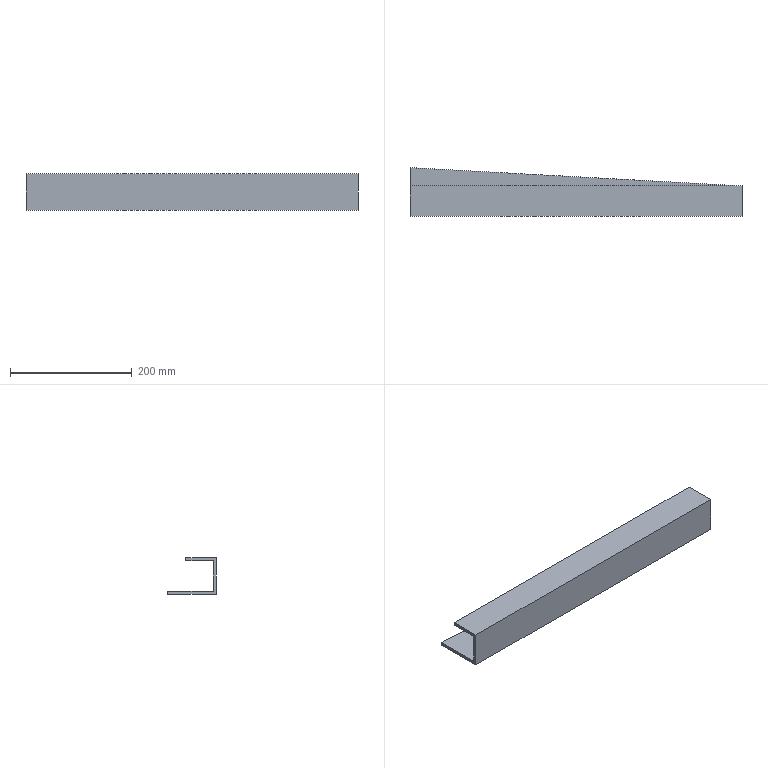Part | SolidWorks | features Extrusion 1, ICE 1, Shell 1 | 1 solid | 10 faces | box 545 x 80 x 60 mm | volume 449625 mm3 | plane 10
STEP:
#1=CARTESIAN_POINT('',(545.,-30.,5.));
#2=VERTEX_POINT('',#1);
#3=CARTESIAN_POINT('',(0.,0.,5.));
#4=VERTEX_POINT('',#3);
#5=CARTESIAN_POINT('',(545.,-30.,5.));
#6=DIRECTION('',(-0.9985,0.05496,0.));
#7=VECTOR('',#6,1000.);
#8=LINE('',#5,#7);
#9=EDGE_CURVE('',#2,#4,#8,.T.);
#10=ORIENTED_EDGE('',*,*,#9,.F.);
#11=CARTESIAN_POINT('',(545.,-30.,0.));
#12=VERTEX_POINT('',#11);
#13=CARTESIAN_POINT('',(545.,-30.,60.));
#14=DIRECTION('',(0.,0.,-1.));
#15=VECTOR('',#14,1000.);
#16=LINE('',#13,#15);
#17=EDGE_CURVE('',#2,#12,#16,.T.);
#18=ORIENTED_EDGE('',*,*,#17,.T.);
#19=CARTESIAN_POINT('',(0.,0.,0.));
#20=VERTEX_POINT('',#19);
#21=CARTESIAN_POINT('',(545.,-30.,0.));
#22=DIRECTION('',(-0.9985,0.05496,0.));
#23=VECTOR('',#22,1000.);
#24=LINE('',#21,#23);
#25=EDGE_CURVE('',#12,#20,#24,.T.);
#26=ORIENTED_EDGE('',*,*,#25,.T.);
#27=CARTESIAN_POINT('',(0.,0.,60.));
#28=DIRECTION('',(0.,0.,-1.));
#29=VECTOR('',#28,1000.);
#30=LINE('',#27,#29);
#31=EDGE_CURVE('',#4,#20,#30,.T.);
#32=ORIENTED_EDGE('',*,*,#31,.F.);
#33=EDGE_LOOP('',(#10,#18,#26,#32));
#34=FACE_OUTER_BOUND('',#33,.T.);
#35=CARTESIAN_POINT('',(545.,-30.,60.));
#36=DIRECTION('',(-0.05496,-0.9985,0.));
#37=DIRECTION('',(0.9985,-0.05496,0.));
#38=AXIS2_PLACEMENT_3D('',#35,#36,#37);
#39=PLANE('',#38);
#40=ADVANCED_FACE('',(#34),#39,.F.);
#41=CARTESIAN_POINT('',(0.,-30.,60.));
#42=VERTEX_POINT('',#41);
#43=CARTESIAN_POINT('',(0.,-80.,60.));
#44=VERTEX_POINT('',#43);
#45=CARTESIAN_POINT('',(0.,0.,60.));
#46=DIRECTION('',(0.,-1.,0.));
#47=VECTOR('',#46,1000.);
#48=LINE('',#45,#47);
#49=EDGE_CURVE('',#42,#44,#48,.T.);
#50=ORIENTED_EDGE('',*,*,#49,.F.);
#51=CARTESIAN_POINT('',(0.,-30.,55.));
#52=VERTEX_POINT('',#51);
#53=CARTESIAN_POINT('',(0.,-30.,22.));
#54=DIRECTION('',(0.,0.,1.));
#55=VECTOR('',#54,1000.);
#56=LINE('',#53,#55);
#57=EDGE_CURVE('',#52,#42,#56,.T.);
#58=ORIENTED_EDGE('',*,*,#57,.F.);
#59=CARTESIAN_POINT('',(0.,-75.,55.));
#60=VERTEX_POINT('',#59);
#61=CARTESIAN_POINT('',(0.,0.,55.));
#62=DIRECTION('',(0.,-1.,0.));
#63=VECTOR('',#62,1000.);
#64=LINE('',#61,#63);
#65=EDGE_CURVE('',#52,#60,#64,.T.);
#66=ORIENTED_EDGE('',*,*,#65,.T.);
#67=CARTESIAN_POINT('',(0.,-75.,5.));
#68=VERTEX_POINT('',#67);
#69=CARTESIAN_POINT('',(0.,-75.,60.));
#70=DIRECTION('',(0.,0.,-1.));
#71=VECTOR('',#70,1000.);
#72=LINE('',#69,#71);
#73=EDGE_CURVE('',#60,#68,#72,.T.);
#74=ORIENTED_EDGE('',*,*,#73,.T.);
#75=CARTESIAN_POINT('',(0.,0.,5.));
#76=DIRECTION('',(0.,-1.,0.));
#77=VECTOR('',#76,1000.);
#78=LINE('',#75,#77);
#79=EDGE_CURVE('',#4,#68,#78,.T.);
#80=ORIENTED_EDGE('',*,*,#79,.F.);
#81=ORIENTED_EDGE('',*,*,#31,.T.);
#82=CARTESIAN_POINT('',(0.,-80.,0.));
#83=VERTEX_POINT('',#82);
#84=CARTESIAN_POINT('',(0.,0.,0.));
#85=DIRECTION('',(0.,-1.,0.));
#86=VECTOR('',#85,1000.);
#87=LINE('',#84,#86);
#88=EDGE_CURVE('',#20,#83,#87,.T.);
#89=ORIENTED_EDGE('',*,*,#88,.T.);
#90=CARTESIAN_POINT('',(0.,-80.,60.));
#91=DIRECTION('',(0.,0.,-1.));
#92=VECTOR('',#91,1000.);
#93=LINE('',#90,#92);
#94=EDGE_CURVE('',#44,#83,#93,.T.);
#95=ORIENTED_EDGE('',*,*,#94,.F.);
#96=EDGE_LOOP('',(#50,#58,#66,#74,#80,#81,#89,#95));
#97=FACE_OUTER_BOUND('',#96,.T.);
#98=CARTESIAN_POINT('',(0.,0.,60.));
#99=DIRECTION('',(1.,0.,0.));
#100=DIRECTION('',(0.,1.,0.));
#101=AXIS2_PLACEMENT_3D('',#98,#99,#100);
#102=PLANE('',#101);
#103=ADVANCED_FACE('',(#97),#102,.F.);
#104=CARTESIAN_POINT('',(545.,-75.,5.));
#105=VERTEX_POINT('',#104);
#106=CARTESIAN_POINT('',(545.,-80.,5.));
#107=DIRECTION('',(0.,1.,0.));
#108=VECTOR('',#107,1000.);
#109=LINE('',#106,#108);
#110=EDGE_CURVE('',#105,#2,#109,.T.);
#111=ORIENTED_EDGE('',*,*,#110,.F.);
#112=CARTESIAN_POINT('',(545.,-75.,55.));
#113=VERTEX_POINT('',#112);
#114=CARTESIAN_POINT('',(545.,-75.,60.));
#115=DIRECTION('',(0.,0.,-1.));
#116=VECTOR('',#115,1000.);
#117=LINE('',#114,#116);
#118=EDGE_CURVE('',#113,#105,#117,.T.);
#119=ORIENTED_EDGE('',*,*,#118,.F.);
#120=CARTESIAN_POINT('',(545.,-30.,55.));
#121=VERTEX_POINT('',#120);
#122=CARTESIAN_POINT('',(545.,-80.,55.));
#123=DIRECTION('',(0.,1.,0.));
#124=VECTOR('',#123,1000.);
#125=LINE('',#122,#124);
#126=EDGE_CURVE('',#113,#121,#125,.T.);
#127=ORIENTED_EDGE('',*,*,#126,.T.);
#128=CARTESIAN_POINT('',(545.,-30.,60.));
#129=VERTEX_POINT('',#128);
#130=CARTESIAN_POINT('',(545.,-30.,60.));
#131=DIRECTION('',(0.,0.,-1.));
#132=VECTOR('',#131,1000.);
#133=LINE('',#130,#132);
#134=EDGE_CURVE('',#129,#121,#133,.T.);
#135=ORIENTED_EDGE('',*,*,#134,.F.);
#136=CARTESIAN_POINT('',(545.,-80.,60.));
#137=VERTEX_POINT('',#136);
#138=CARTESIAN_POINT('',(545.,-80.,60.));
#139=DIRECTION('',(0.,1.,0.));
#140=VECTOR('',#139,1000.);
#141=LINE('',#138,#140);
#142=EDGE_CURVE('',#137,#129,#141,.T.);
#143=ORIENTED_EDGE('',*,*,#142,.F.);
#144=CARTESIAN_POINT('',(545.,-80.,0.));
#145=VERTEX_POINT('',#144);
#146=CARTESIAN_POINT('',(545.,-80.,60.));
#147=DIRECTION('',(0.,0.,-1.));
#148=VECTOR('',#147,1000.);
#149=LINE('',#146,#148);
#150=EDGE_CURVE('',#137,#145,#149,.T.);
#151=ORIENTED_EDGE('',*,*,#150,.T.);
#152=CARTESIAN_POINT('',(545.,-80.,0.));
#153=DIRECTION('',(0.,1.,0.));
#154=VECTOR('',#153,1000.);
#155=LINE('',#152,#154);
#156=EDGE_CURVE('',#145,#12,#155,.T.);
#157=ORIENTED_EDGE('',*,*,#156,.T.);
#158=ORIENTED_EDGE('',*,*,#17,.F.);
#159=EDGE_LOOP('',(#111,#119,#127,#135,#143,#151,#157,#158));
#160=FACE_OUTER_BOUND('',#159,.T.);
#161=CARTESIAN_POINT('',(545.,-80.,60.));
#162=DIRECTION('',(-1.,0.,0.));
#163=DIRECTION('',(0.,0.,1.));
#164=AXIS2_PLACEMENT_3D('',#161,#162,#163);
#165=PLANE('',#164);
#166=ADVANCED_FACE('',(#160),#165,.F.);
#167=CARTESIAN_POINT('',(0.,-80.,0.));
#168=DIRECTION('',(1.,0.,0.));
#169=VECTOR('',#168,1000.);
#170=LINE('',#167,#169);
#171=EDGE_CURVE('',#83,#145,#170,.T.);
#172=ORIENTED_EDGE('',*,*,#171,.T.);
#173=ORIENTED_EDGE('',*,*,#150,.F.);
#174=CARTESIAN_POINT('',(0.,-80.,60.));
#175=DIRECTION('',(1.,0.,0.));
#176=VECTOR('',#175,1000.);
#177=LINE('',#174,#176);
#178=EDGE_CURVE('',#44,#137,#177,.T.);
#179=ORIENTED_EDGE('',*,*,#178,.F.);
#180=ORIENTED_EDGE('',*,*,#94,.T.);
#181=EDGE_LOOP('',(#172,#173,#179,#180));
#182=FACE_OUTER_BOUND('',#181,.T.);
#183=CARTESIAN_POINT('',(0.,-80.,60.));
#184=DIRECTION('',(0.,1.,0.));
#185=DIRECTION('',(0.,0.,1.));
#186=AXIS2_PLACEMENT_3D('',#183,#184,#185);
#187=PLANE('',#186);
#188=ADVANCED_FACE('',(#182),#187,.F.);
#189=CARTESIAN_POINT('',(545.,-30.,60.));
#190=DIRECTION('',(1.,0.,0.));
#191=VECTOR('',#190,1000.);
#192=LINE('',#189,#191);
#193=EDGE_CURVE('',#42,#129,#192,.T.);
#194=ORIENTED_EDGE('',*,*,#193,.F.);
#195=ORIENTED_EDGE('',*,*,#49,.T.);
#196=ORIENTED_EDGE('',*,*,#178,.T.);
#197=ORIENTED_EDGE('',*,*,#142,.T.);
#198=EDGE_LOOP('',(#194,#195,#196,#197));
#199=FACE_OUTER_BOUND('',#198,.T.);
#200=CARTESIAN_POINT('',(0.,0.,60.));
#201=DIRECTION('',(0.,0.,1.));
#202=DIRECTION('',(1.,0.,0.));
#203=AXIS2_PLACEMENT_3D('',#200,#201,#202);
#204=PLANE('',#203);
#205=ADVANCED_FACE('',(#199),#204,.T.);
#206=ORIENTED_EDGE('',*,*,#25,.F.);
#207=ORIENTED_EDGE('',*,*,#156,.F.);
#208=ORIENTED_EDGE('',*,*,#171,.F.);
#209=ORIENTED_EDGE('',*,*,#88,.F.);
#210=EDGE_LOOP('',(#206,#207,#208,#209));
#211=FACE_OUTER_BOUND('',#210,.T.);
#212=CARTESIAN_POINT('',(0.,0.,0.));
#213=DIRECTION('',(0.,0.,1.));
#214=DIRECTION('',(1.,0.,0.));
#215=AXIS2_PLACEMENT_3D('',#212,#213,#214);
#216=PLANE('',#215);
#217=ADVANCED_FACE('',(#211),#216,.F.);
#218=CARTESIAN_POINT('',(0.,-75.,5.));
#219=DIRECTION('',(1.,0.,0.));
#220=VECTOR('',#219,1000.);
#221=LINE('',#218,#220);
#222=EDGE_CURVE('',#68,#105,#221,.T.);
#223=ORIENTED_EDGE('',*,*,#222,.F.);
#224=ORIENTED_EDGE('',*,*,#73,.F.);
#225=CARTESIAN_POINT('',(0.,-75.,55.));
#226=DIRECTION('',(1.,0.,0.));
#227=VECTOR('',#226,1000.);
#228=LINE('',#225,#227);
#229=EDGE_CURVE('',#60,#113,#228,.T.);
#230=ORIENTED_EDGE('',*,*,#229,.T.);
#231=ORIENTED_EDGE('',*,*,#118,.T.);
#232=EDGE_LOOP('',(#223,#224,#230,#231));
#233=FACE_OUTER_BOUND('',#232,.T.);
#234=CARTESIAN_POINT('',(0.,-75.,60.));
#235=DIRECTION('',(0.,1.,0.));
#236=DIRECTION('',(0.,0.,1.));
#237=AXIS2_PLACEMENT_3D('',#234,#235,#236);
#238=PLANE('',#237);
#239=ADVANCED_FACE('',(#233),#238,.T.);
#240=ORIENTED_EDGE('',*,*,#65,.F.);
#241=CARTESIAN_POINT('',(0.,-30.,55.));
#242=DIRECTION('',(1.,0.,0.));
#243=VECTOR('',#242,1000.);
#244=LINE('',#241,#243);
#245=EDGE_CURVE('',#52,#121,#244,.T.);
#246=ORIENTED_EDGE('',*,*,#245,.T.);
#247=ORIENTED_EDGE('',*,*,#126,.F.);
#248=ORIENTED_EDGE('',*,*,#229,.F.);
#249=EDGE_LOOP('',(#240,#246,#247,#248));
#250=FACE_OUTER_BOUND('',#249,.T.);
#251=CARTESIAN_POINT('',(0.,0.,55.));
#252=DIRECTION('',(0.,0.,1.));
#253=DIRECTION('',(1.,0.,0.));
#254=AXIS2_PLACEMENT_3D('',#251,#252,#253);
#255=PLANE('',#254);
#256=ADVANCED_FACE('',(#250),#255,.F.);
#257=ORIENTED_EDGE('',*,*,#9,.T.);
#258=ORIENTED_EDGE('',*,*,#79,.T.);
#259=ORIENTED_EDGE('',*,*,#222,.T.);
#260=ORIENTED_EDGE('',*,*,#110,.T.);
#261=EDGE_LOOP('',(#257,#258,#259,#260));
#262=FACE_OUTER_BOUND('',#261,.T.);
#263=CARTESIAN_POINT('',(0.,0.,5.));
#264=DIRECTION('',(0.,0.,1.));
#265=DIRECTION('',(1.,0.,0.));
#266=AXIS2_PLACEMENT_3D('',#263,#264,#265);
#267=PLANE('',#266);
#268=ADVANCED_FACE('',(#262),#267,.T.);
#269=ORIENTED_EDGE('',*,*,#57,.T.);
#270=ORIENTED_EDGE('',*,*,#193,.T.);
#271=ORIENTED_EDGE('',*,*,#134,.T.);
#272=ORIENTED_EDGE('',*,*,#245,.F.);
#273=EDGE_LOOP('',(#269,#270,#271,#272));
#274=FACE_OUTER_BOUND('',#273,.T.);
#275=CARTESIAN_POINT('',(545.,-30.,22.));
#276=DIRECTION('',(0.,-1.,0.));
#277=DIRECTION('',(0.,0.,-1.));
#278=AXIS2_PLACEMENT_3D('',#275,#276,#277);
#279=PLANE('',#278);
#280=ADVANCED_FACE('',(#274),#279,.F.);
#281=CLOSED_SHELL('',(#40,#103,#166,#188,#205,#217,#239,#256,#268,#280));
#282=MANIFOLD_SOLID_BREP('',#281);
#283=CARTESIAN_POINT('',(0.,0.,0.));
#284=DIRECTION('',(0.,0.,1.));
#285=DIRECTION('',(1.,0.,0.));
#286=AXIS2_PLACEMENT_3D('',#283,#284,#285);
#287=(LENGTH_UNIT()NAMED_UNIT(*)SI_UNIT(.MILLI.,.METRE.));
#288=UNCERTAINTY_MEASURE_WITH_UNIT(LENGTH_MEASURE(0.00001),#287,'','');
#289=(NAMED_UNIT(*)PLANE_ANGLE_UNIT()SI_UNIT($,.RADIAN.));
#290=(NAMED_UNIT(*)SI_UNIT($,.STERADIAN.)SOLID_ANGLE_UNIT());
#291=(GEOMETRIC_REPRESENTATION_CONTEXT(3)GLOBAL_UNCERTAINTY_ASSIGNED_CONTEXT((#288))GLOBAL_UNIT_ASSIGNED_CONTEXT((#287,#289,#290))REPRESENTATION_CONTEXT('',''));
#292=ADVANCED_BREP_SHAPE_REPRESENTATION('',(#282,#286),#291);